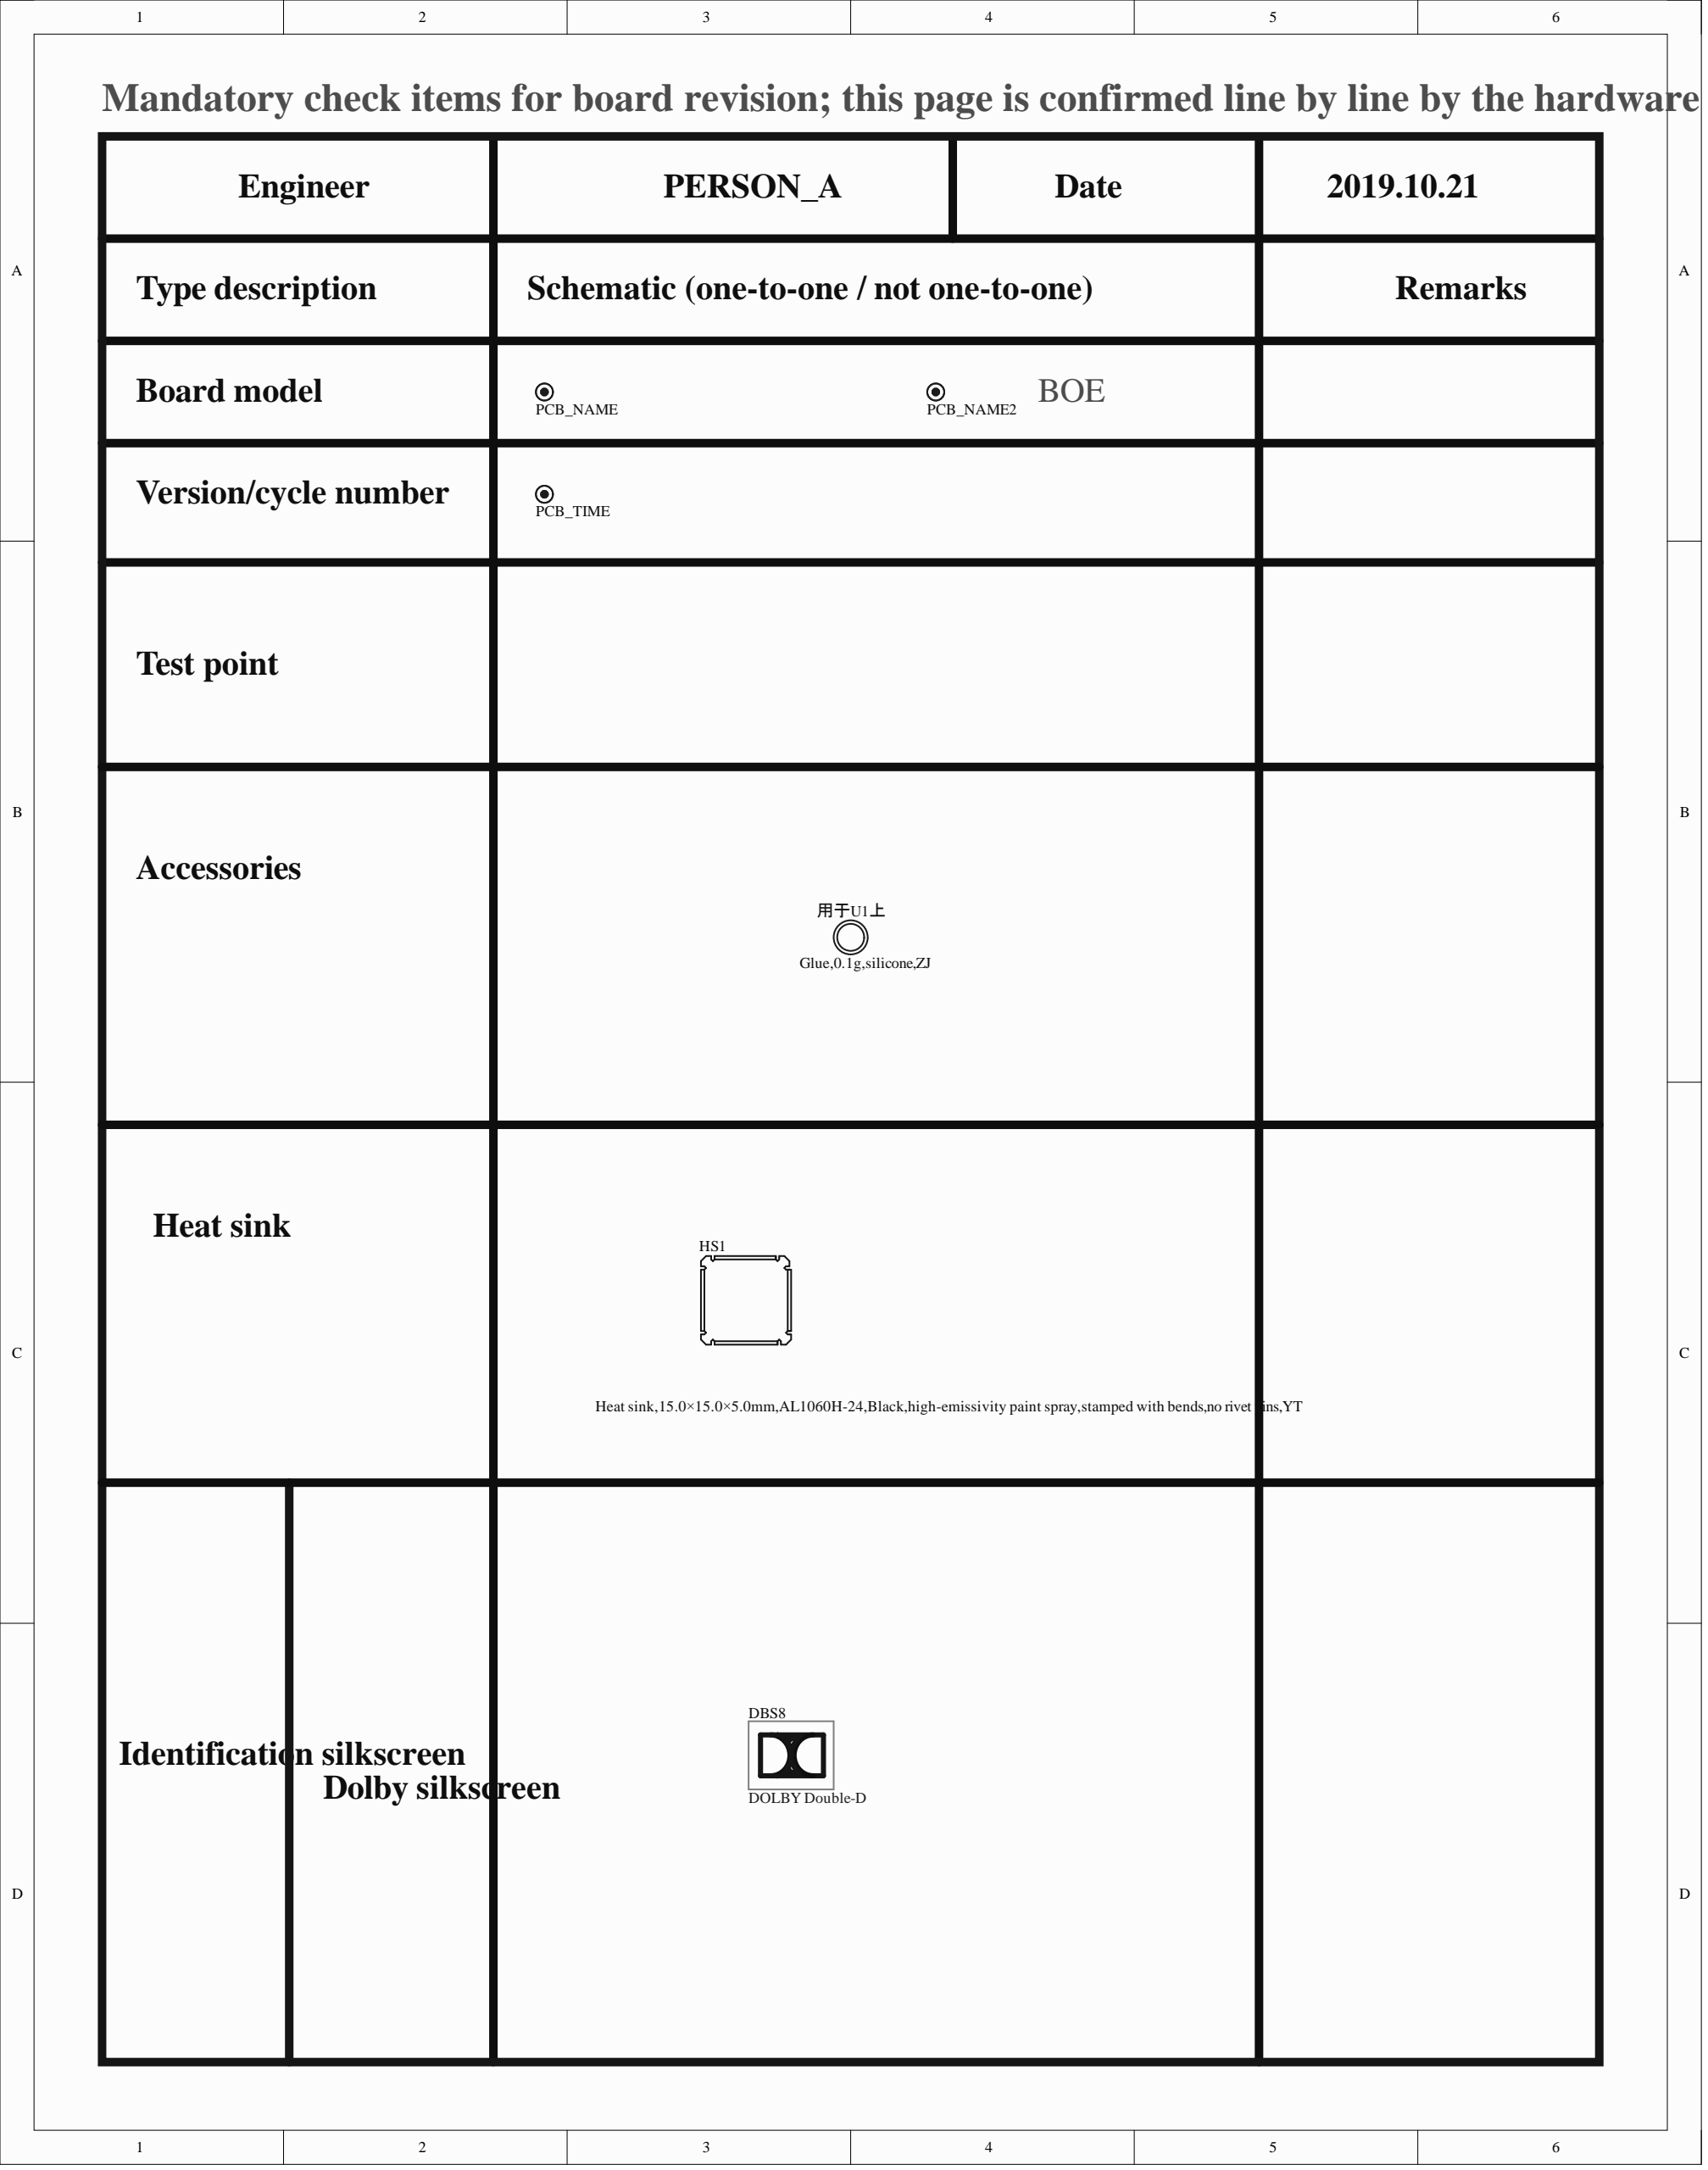Circuit board | Altium Designer | 527 parts | 243 nets | one sheet of the schematic
Parts on this sheet (reference | value | footprint):
BOE | PCB_NAME2 | PCB_NAME
DBS8 | DOLBY Double-D | Double-D-SILK
HS1 | Heat sink,15.0×15.0×5.0mm,AL1060H-24,Black,high-emissivity paint spray,stamped with bends,no rivet pins,YT | HS(15X15X5)-S
用于U1上 | Glue,0.1g,silicone,ZJ | Heat-Shrinkable Tube
Nets of these parts (net: part-pin ...):